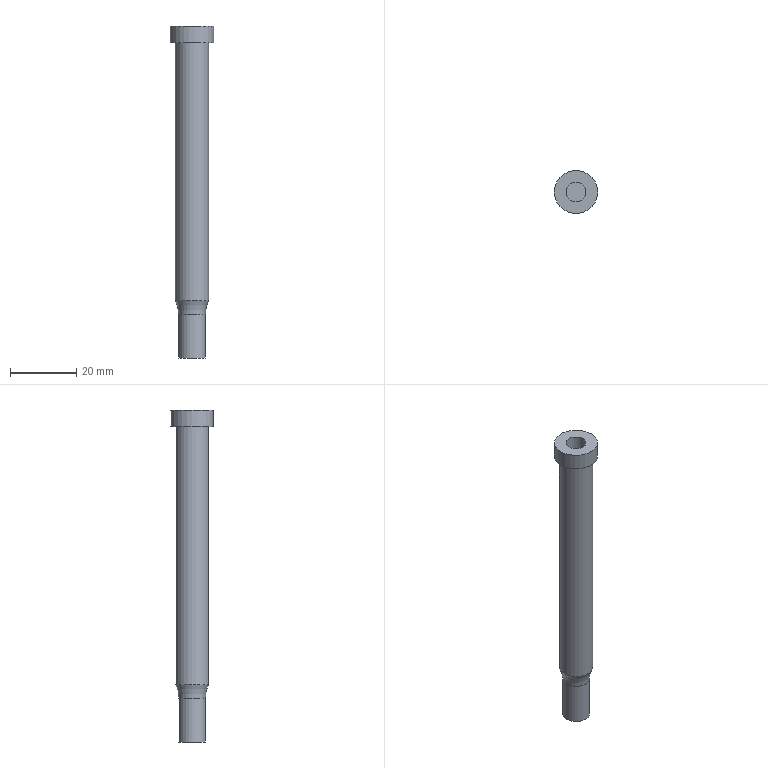Part | NX | features SPAS-C 10-80-8.100 2 | 1 solid | 9 faces | box 13 x 13 x 100 mm | volume 6762 mm3 | plane 4 | cylinder 4 | torus 1 | commonest cylinder face diameters 6 x1 8.1 x1 10 x1 13 x1
STEP:
#1=CARTESIAN_POINT('',(688.638,-2.702,-10.));
#2=VERTEX_POINT('',#1);
#3=CARTESIAN_POINT('',(684.588,-2.702,-10.));
#4=DIRECTION('',(0.,0.,1.));
#5=DIRECTION('',(1.,0.,0.));
#6=AXIS2_PLACEMENT_3D('',#3,#4,#5);
#7=CIRCLE('',#6,4.05);
#8=EDGE_CURVE('',#2,#2,#7,.T.);
#9=ORIENTED_EDGE('',*,*,#8,.F.);
#10=EDGE_LOOP('',(#9));
#11=FACE_BOUND('',#10,.T.);
#12=CARTESIAN_POINT('',(684.588,-2.702,-10.));
#13=DIRECTION('',(0.,0.,-1.));
#14=DIRECTION('',(-1.,0.,0.));
#15=AXIS2_PLACEMENT_3D('',#12,#13,#14);
#16=PLANE('',#15);
#17=ADVANCED_FACE('',(#11),#16,.T.);
#18=CARTESIAN_POINT('',(688.638,-2.702,3.));
#19=VERTEX_POINT('',#18);
#20=CARTESIAN_POINT('',(684.588,-2.702,3.));
#21=DIRECTION('',(0.,0.,1.));
#22=DIRECTION('',(1.,0.,0.));
#23=AXIS2_PLACEMENT_3D('',#20,#21,#22);
#24=CIRCLE('',#23,4.05);
#25=EDGE_CURVE('',#19,#19,#24,.F.);
#26=ORIENTED_EDGE('',*,*,#25,.T.);
#27=EDGE_LOOP('',(#26));
#28=FACE_BOUND('',#27,.T.);
#29=ORIENTED_EDGE('',*,*,#8,.T.);
#30=EDGE_LOOP('',(#29));
#31=FACE_BOUND('',#30,.T.);
#32=CARTESIAN_POINT('',(684.588,-2.702,-10.));
#33=DIRECTION('',(0.,0.,1.));
#34=DIRECTION('',(1.,0.,0.));
#35=AXIS2_PLACEMENT_3D('',#32,#33,#34);
#36=CYLINDRICAL_SURFACE('',#35,4.05);
#37=ADVANCED_FACE('',(#28,#31),#36,.T.);
#38=CARTESIAN_POINT('',(679.588,-2.702,85.));
#39=VERTEX_POINT('',#38);
#40=CARTESIAN_POINT('',(684.588,-2.702,85.));
#41=DIRECTION('',(0.,0.,-1.));
#42=DIRECTION('',(-1.,0.,0.));
#43=AXIS2_PLACEMENT_3D('',#40,#41,#42);
#44=CIRCLE('',#43,5.);
#45=EDGE_CURVE('',#39,#39,#44,.F.);
#46=ORIENTED_EDGE('',*,*,#45,.F.);
#47=EDGE_LOOP('',(#46));
#48=FACE_BOUND('',#47,.T.);
#49=CARTESIAN_POINT('',(689.588,-2.702,7.254));
#50=VERTEX_POINT('',#49);
#51=CARTESIAN_POINT('',(684.588,-2.702,7.254));
#52=DIRECTION('',(0.,0.,1.));
#53=DIRECTION('',(1.,0.,0.));
#54=AXIS2_PLACEMENT_3D('',#51,#52,#53);
#55=CIRCLE('',#54,5.);
#56=EDGE_CURVE('',#50,#50,#55,.T.);
#57=ORIENTED_EDGE('',*,*,#56,.T.);
#58=EDGE_LOOP('',(#57));
#59=FACE_BOUND('',#58,.T.);
#60=CARTESIAN_POINT('',(684.588,-2.702,7.254));
#61=DIRECTION('',(0.,0.,1.));
#62=DIRECTION('',(1.,0.,0.));
#63=AXIS2_PLACEMENT_3D('',#60,#61,#62);
#64=CYLINDRICAL_SURFACE('',#63,5.);
#65=ADVANCED_FACE('',(#48,#59),#64,.T.);
#66=CARTESIAN_POINT('',(687.588,-2.702,90.));
#67=VERTEX_POINT('',#66);
#68=CARTESIAN_POINT('',(684.588,-2.702,90.));
#69=DIRECTION('',(0.,0.,1.));
#70=DIRECTION('',(1.,0.,0.));
#71=AXIS2_PLACEMENT_3D('',#68,#69,#70);
#72=CIRCLE('',#71,3.);
#73=EDGE_CURVE('',#67,#67,#72,.T.);
#74=ORIENTED_EDGE('',*,*,#73,.F.);
#75=EDGE_LOOP('',(#74));
#76=FACE_BOUND('',#75,.T.);
#77=CARTESIAN_POINT('',(691.088,-2.702,90.));
#78=VERTEX_POINT('',#77);
#79=CARTESIAN_POINT('',(684.588,-2.702,90.));
#80=DIRECTION('',(0.,0.,1.));
#81=DIRECTION('',(1.,0.,0.));
#82=AXIS2_PLACEMENT_3D('',#79,#80,#81);
#83=CIRCLE('',#82,6.5);
#84=EDGE_CURVE('',#78,#78,#83,.F.);
#85=ORIENTED_EDGE('',*,*,#84,.F.);
#86=EDGE_LOOP('',(#85));
#87=FACE_BOUND('',#86,.T.);
#88=CARTESIAN_POINT('',(684.588,-2.702,90.));
#89=DIRECTION('',(0.,0.,1.));
#90=DIRECTION('',(1.,0.,0.));
#91=AXIS2_PLACEMENT_3D('',#88,#89,#90);
#92=PLANE('',#91);
#93=ADVANCED_FACE('',(#76,#87),#92,.T.);
#94=ORIENTED_EDGE('',*,*,#45,.T.);
#95=EDGE_LOOP('',(#94));
#96=FACE_BOUND('',#95,.T.);
#97=CARTESIAN_POINT('',(678.088,-2.702,85.));
#98=VERTEX_POINT('',#97);
#99=CARTESIAN_POINT('',(684.588,-2.702,85.));
#100=DIRECTION('',(0.,0.,-1.));
#101=DIRECTION('',(-1.,0.,0.));
#102=AXIS2_PLACEMENT_3D('',#99,#100,#101);
#103=CIRCLE('',#102,6.5);
#104=EDGE_CURVE('',#98,#98,#103,.F.);
#105=ORIENTED_EDGE('',*,*,#104,.F.);
#106=EDGE_LOOP('',(#105));
#107=FACE_BOUND('',#106,.T.);
#108=CARTESIAN_POINT('',(684.588,-2.702,85.));
#109=DIRECTION('',(0.,0.,-1.));
#110=DIRECTION('',(-1.,0.,0.));
#111=AXIS2_PLACEMENT_3D('',#108,#109,#110);
#112=PLANE('',#111);
#113=ADVANCED_FACE('',(#96,#107),#112,.T.);
#114=ORIENTED_EDGE('',*,*,#84,.T.);
#115=EDGE_LOOP('',(#114));
#116=FACE_BOUND('',#115,.T.);
#117=ORIENTED_EDGE('',*,*,#104,.T.);
#118=EDGE_LOOP('',(#117));
#119=FACE_BOUND('',#118,.T.);
#120=CARTESIAN_POINT('',(684.588,-2.702,65.));
#121=DIRECTION('',(0.,0.,1.));
#122=DIRECTION('',(1.,0.,0.));
#123=AXIS2_PLACEMENT_3D('',#120,#121,#122);
#124=CYLINDRICAL_SURFACE('',#123,6.5);
#125=ADVANCED_FACE('',(#116,#119),#124,.T.);
#126=CARTESIAN_POINT('',(687.588,-2.702,57.));
#127=VERTEX_POINT('',#126);
#128=CARTESIAN_POINT('',(684.588,-2.702,57.));
#129=DIRECTION('',(0.,0.,1.));
#130=DIRECTION('',(1.,0.,0.));
#131=AXIS2_PLACEMENT_3D('',#128,#129,#130);
#132=CIRCLE('',#131,3.);
#133=EDGE_CURVE('',#127,#127,#132,.T.);
#134=ORIENTED_EDGE('',*,*,#133,.T.);
#135=EDGE_LOOP('',(#134));
#136=FACE_BOUND('',#135,.T.);
#137=CARTESIAN_POINT('',(684.588,-2.702,57.));
#138=DIRECTION('',(0.,0.,-1.));
#139=DIRECTION('',(-1.,0.,0.));
#140=AXIS2_PLACEMENT_3D('',#137,#138,#139);
#141=PLANE('',#140);
#142=ADVANCED_FACE('',(#136),#141,.F.);
#143=ORIENTED_EDGE('',*,*,#73,.T.);
#144=EDGE_LOOP('',(#143));
#145=FACE_BOUND('',#144,.T.);
#146=ORIENTED_EDGE('',*,*,#133,.F.);
#147=EDGE_LOOP('',(#146));
#148=FACE_BOUND('',#147,.T.);
#149=CARTESIAN_POINT('',(684.588,-2.702,57.));
#150=DIRECTION('',(0.,0.,1.));
#151=DIRECTION('',(1.,0.,0.));
#152=AXIS2_PLACEMENT_3D('',#149,#150,#151);
#153=CYLINDRICAL_SURFACE('',#152,3.);
#154=ADVANCED_FACE('',(#145,#148),#153,.F.);
#155=ORIENTED_EDGE('',*,*,#25,.F.);
#156=EDGE_LOOP('',(#155));
#157=FACE_BOUND('',#156,.T.);
#158=ORIENTED_EDGE('',*,*,#56,.F.);
#159=EDGE_LOOP('',(#158));
#160=FACE_BOUND('',#159,.T.);
#161=CARTESIAN_POINT('',(684.588,-2.702,3.));
#162=DIRECTION('',(0.,0.,1.));
#163=DIRECTION('',(1.,0.,0.));
#164=AXIS2_PLACEMENT_3D('',#161,#162,#163);
#165=TOROIDAL_SURFACE('',#164,14.05,10.);
#166=ADVANCED_FACE('',(#157,#160),#165,.F.);
#167=CLOSED_SHELL('',(#17,#37,#65,#93,#113,#125,#142,#154,#166));
#168=MANIFOLD_SOLID_BREP('',#167);
#169=(LENGTH_UNIT()NAMED_UNIT(*)SI_UNIT(.MILLI.,.METRE.));
#170=UNCERTAINTY_MEASURE_WITH_UNIT(LENGTH_MEASURE(0.00001),#169,'','');
#171=(NAMED_UNIT(*)PLANE_ANGLE_UNIT()SI_UNIT($,.RADIAN.));
#172=(NAMED_UNIT(*)SI_UNIT($,.STERADIAN.)SOLID_ANGLE_UNIT());
#173=(GEOMETRIC_REPRESENTATION_CONTEXT(3)GLOBAL_UNCERTAINTY_ASSIGNED_CONTEXT((#170))GLOBAL_UNIT_ASSIGNED_CONTEXT((#169,#171,#172))REPRESENTATION_CONTEXT('',''));
#174=ADVANCED_BREP_SHAPE_REPRESENTATION('',(#168),#173);